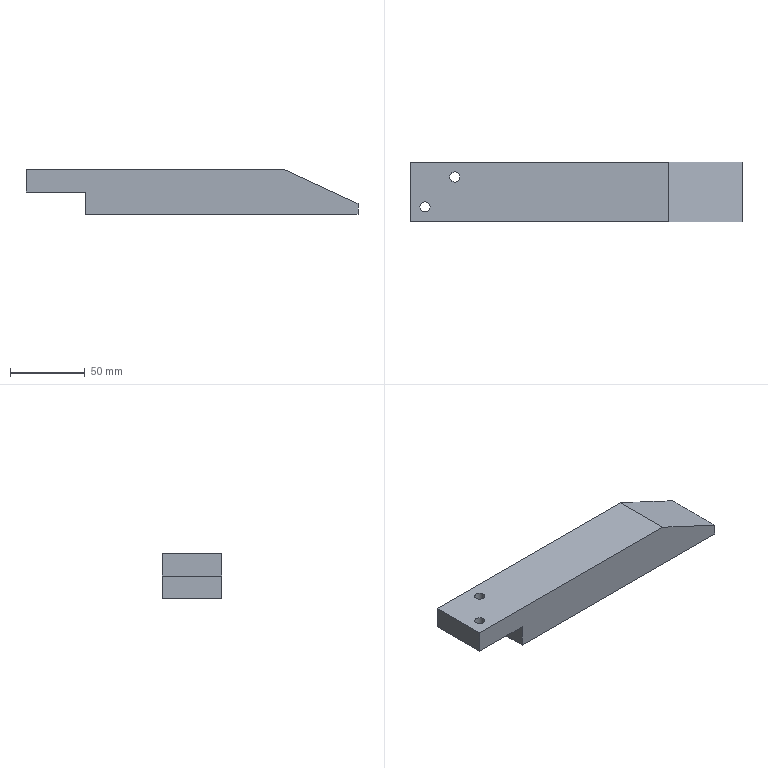Part | NX | features solid 2 | 1 solid | 11 faces | box 222 x 40 x 30 mm | volume 219063 mm3 | plane 9 | cylinder 2 | commonest cylinder face diameters 6.8 x2
STEP:
#1=CARTESIAN_POINT('',(3424.4,108.,-48.5));
#2=VERTEX_POINT('',#1);
#3=CARTESIAN_POINT('',(3421.,108.,-48.5));
#4=DIRECTION('',(0.,0.,1.));
#5=DIRECTION('',(1.,0.,0.));
#6=AXIS2_PLACEMENT_3D('',#3,#4,#5);
#7=CIRCLE('',#6,3.4);
#8=EDGE_CURVE('',#2,#2,#7,.T.);
#9=ORIENTED_EDGE('',*,*,#8,.T.);
#10=EDGE_LOOP('',(#9));
#11=FACE_BOUND('',#10,.T.);
#12=CARTESIAN_POINT('',(3444.4,128.,-48.5));
#13=VERTEX_POINT('',#12);
#14=CARTESIAN_POINT('',(3441.,128.,-48.5));
#15=DIRECTION('',(0.,0.,1.));
#16=DIRECTION('',(1.,0.,0.));
#17=AXIS2_PLACEMENT_3D('',#14,#15,#16);
#18=CIRCLE('',#17,3.4);
#19=EDGE_CURVE('',#13,#13,#18,.T.);
#20=ORIENTED_EDGE('',*,*,#19,.T.);
#21=EDGE_LOOP('',(#20));
#22=FACE_BOUND('',#21,.T.);
#23=CARTESIAN_POINT('',(3451.,138.,-48.5));
#24=VERTEX_POINT('',#23);
#25=CARTESIAN_POINT('',(3451.,98.,-48.5));
#26=VERTEX_POINT('',#25);
#27=CARTESIAN_POINT('',(3451.,0.,-48.5));
#28=DIRECTION('',(0.,-1.,0.));
#29=VECTOR('',#28,1000.);
#30=LINE('',#27,#29);
#31=EDGE_CURVE('',#24,#26,#30,.T.);
#32=ORIENTED_EDGE('',*,*,#31,.T.);
#33=CARTESIAN_POINT('',(3411.,98.,-48.5));
#34=VERTEX_POINT('',#33);
#35=CARTESIAN_POINT('',(3699.,98.,-48.5));
#36=DIRECTION('',(1.,0.,0.));
#37=VECTOR('',#36,1000.);
#38=LINE('',#35,#37);
#39=EDGE_CURVE('',#34,#26,#38,.T.);
#40=ORIENTED_EDGE('',*,*,#39,.F.);
#41=CARTESIAN_POINT('',(3411.,138.,-48.5));
#42=VERTEX_POINT('',#41);
#43=CARTESIAN_POINT('',(3411.,0.,-48.5));
#44=DIRECTION('',(0.,1.,0.));
#45=VECTOR('',#44,1000.);
#46=LINE('',#43,#45);
#47=EDGE_CURVE('',#34,#42,#46,.T.);
#48=ORIENTED_EDGE('',*,*,#47,.T.);
#49=CARTESIAN_POINT('',(3699.,138.,-48.5));
#50=DIRECTION('',(1.,0.,0.));
#51=VECTOR('',#50,1000.);
#52=LINE('',#49,#51);
#53=EDGE_CURVE('',#42,#24,#52,.T.);
#54=ORIENTED_EDGE('',*,*,#53,.T.);
#55=EDGE_LOOP('',(#32,#40,#48,#54));
#56=FACE_BOUND('',#55,.T.);
#57=CARTESIAN_POINT('',(3411.,138.,-48.5));
#58=DIRECTION('',(0.,0.,1.));
#59=DIRECTION('',(-1.,0.,0.));
#60=AXIS2_PLACEMENT_3D('',#57,#58,#59);
#61=PLANE('',#60);
#62=ADVANCED_FACE('',(#11,#22,#56),#61,.F.);
#63=CARTESIAN_POINT('',(3424.4,108.,-33.5));
#64=VERTEX_POINT('',#63);
#65=CARTESIAN_POINT('',(3421.,108.,-33.5));
#66=DIRECTION('',(0.,0.,1.));
#67=DIRECTION('',(1.,0.,0.));
#68=AXIS2_PLACEMENT_3D('',#65,#66,#67);
#69=CIRCLE('',#68,3.4);
#70=EDGE_CURVE('',#64,#64,#69,.T.);
#71=ORIENTED_EDGE('',*,*,#70,.F.);
#72=EDGE_LOOP('',(#71));
#73=FACE_BOUND('',#72,.T.);
#74=CARTESIAN_POINT('',(3444.4,128.,-33.5));
#75=VERTEX_POINT('',#74);
#76=CARTESIAN_POINT('',(3441.,128.,-33.5));
#77=DIRECTION('',(0.,0.,1.));
#78=DIRECTION('',(1.,0.,0.));
#79=AXIS2_PLACEMENT_3D('',#76,#77,#78);
#80=CIRCLE('',#79,3.4);
#81=EDGE_CURVE('',#75,#75,#80,.T.);
#82=ORIENTED_EDGE('',*,*,#81,.F.);
#83=EDGE_LOOP('',(#82));
#84=FACE_BOUND('',#83,.T.);
#85=CARTESIAN_POINT('',(3584.159,138.,-33.5));
#86=VERTEX_POINT('',#85);
#87=CARTESIAN_POINT('',(3411.,138.,-33.5));
#88=VERTEX_POINT('',#87);
#89=CARTESIAN_POINT('',(3699.,138.,-33.5));
#90=DIRECTION('',(-1.,0.,0.));
#91=VECTOR('',#90,1000.);
#92=LINE('',#89,#91);
#93=EDGE_CURVE('',#86,#88,#92,.T.);
#94=ORIENTED_EDGE('',*,*,#93,.T.);
#95=CARTESIAN_POINT('',(3411.,98.,-33.5));
#96=VERTEX_POINT('',#95);
#97=CARTESIAN_POINT('',(3411.,0.,-33.5));
#98=DIRECTION('',(0.,-1.,0.));
#99=VECTOR('',#98,1000.);
#100=LINE('',#97,#99);
#101=EDGE_CURVE('',#88,#96,#100,.T.);
#102=ORIENTED_EDGE('',*,*,#101,.T.);
#103=CARTESIAN_POINT('',(3584.159,98.,-33.5));
#104=VERTEX_POINT('',#103);
#105=CARTESIAN_POINT('',(3699.,98.,-33.5));
#106=DIRECTION('',(1.,0.,0.));
#107=VECTOR('',#106,1000.);
#108=LINE('',#105,#107);
#109=EDGE_CURVE('',#96,#104,#108,.T.);
#110=ORIENTED_EDGE('',*,*,#109,.T.);
#111=CARTESIAN_POINT('',(3584.159,118.,-33.5));
#112=DIRECTION('',(0.,-1.,0.));
#113=VECTOR('',#112,1000.);
#114=LINE('',#111,#113);
#115=EDGE_CURVE('',#86,#104,#114,.T.);
#116=ORIENTED_EDGE('',*,*,#115,.F.);
#117=EDGE_LOOP('',(#94,#102,#110,#116));
#118=FACE_BOUND('',#117,.T.);
#119=CARTESIAN_POINT('',(3699.,118.,-33.5));
#120=DIRECTION('',(0.,0.,1.));
#121=DIRECTION('',(-1.,0.,0.));
#122=AXIS2_PLACEMENT_3D('',#119,#120,#121);
#123=PLANE('',#122);
#124=ADVANCED_FACE('',(#73,#84,#118),#123,.T.);
#125=CARTESIAN_POINT('',(3633.,138.,-56.275));
#126=VERTEX_POINT('',#125);
#127=CARTESIAN_POINT('',(3642.615,138.,-60.759));
#128=DIRECTION('',(-0.9063,0.,0.4226));
#129=VECTOR('',#128,1000.);
#130=LINE('',#127,#129);
#131=EDGE_CURVE('',#126,#86,#130,.T.);
#132=ORIENTED_EDGE('',*,*,#131,.T.);
#133=ORIENTED_EDGE('',*,*,#115,.T.);
#134=CARTESIAN_POINT('',(3633.,98.,-56.275));
#135=VERTEX_POINT('',#134);
#136=CARTESIAN_POINT('',(3642.615,98.,-60.759));
#137=DIRECTION('',(0.9063,0.,-0.4226));
#138=VECTOR('',#137,1000.);
#139=LINE('',#136,#138);
#140=EDGE_CURVE('',#104,#135,#139,.T.);
#141=ORIENTED_EDGE('',*,*,#140,.T.);
#142=CARTESIAN_POINT('',(3633.,-27.,-56.275));
#143=DIRECTION('',(0.,1.,0.));
#144=VECTOR('',#143,1000.);
#145=LINE('',#142,#144);
#146=EDGE_CURVE('',#135,#126,#145,.T.);
#147=ORIENTED_EDGE('',*,*,#146,.T.);
#148=EDGE_LOOP('',(#132,#133,#141,#147));
#149=FACE_BOUND('',#148,.T.);
#150=CARTESIAN_POINT('',(3868.932,193.251,-166.292));
#151=DIRECTION('',(0.4226,0.,0.9063));
#152=DIRECTION('',(-0.9063,0.,0.4226));
#153=AXIS2_PLACEMENT_3D('',#150,#151,#152);
#154=PLANE('',#153);
#155=ADVANCED_FACE('',(#149),#154,.T.);
#156=ORIENTED_EDGE('',*,*,#47,.F.);
#157=CARTESIAN_POINT('',(3411.,98.,-53.5));
#158=DIRECTION('',(0.,0.,1.));
#159=VECTOR('',#158,1000.);
#160=LINE('',#157,#159);
#161=EDGE_CURVE('',#34,#96,#160,.T.);
#162=ORIENTED_EDGE('',*,*,#161,.T.);
#163=ORIENTED_EDGE('',*,*,#101,.F.);
#164=CARTESIAN_POINT('',(3411.,138.,-63.5));
#165=DIRECTION('',(0.,0.,1.));
#166=VECTOR('',#165,1000.);
#167=LINE('',#164,#166);
#168=EDGE_CURVE('',#42,#88,#167,.T.);
#169=ORIENTED_EDGE('',*,*,#168,.F.);
#170=EDGE_LOOP('',(#156,#162,#163,#169));
#171=FACE_BOUND('',#170,.T.);
#172=CARTESIAN_POINT('',(3411.,0.,-63.5));
#173=DIRECTION('',(-1.,0.,0.));
#174=DIRECTION('',(0.,0.,-1.));
#175=AXIS2_PLACEMENT_3D('',#172,#173,#174);
#176=PLANE('',#175);
#177=ADVANCED_FACE('',(#171),#176,.T.);
#178=ORIENTED_EDGE('',*,*,#39,.T.);
#179=CARTESIAN_POINT('',(3451.,98.,-63.5));
#180=VERTEX_POINT('',#179);
#181=CARTESIAN_POINT('',(3451.,98.,-53.5));
#182=DIRECTION('',(0.,0.,1.));
#183=VECTOR('',#182,1000.);
#184=LINE('',#181,#183);
#185=EDGE_CURVE('',#180,#26,#184,.T.);
#186=ORIENTED_EDGE('',*,*,#185,.F.);
#187=CARTESIAN_POINT('',(3633.,98.,-63.5));
#188=VERTEX_POINT('',#187);
#189=CARTESIAN_POINT('',(3699.,98.,-63.5));
#190=DIRECTION('',(-1.,0.,0.));
#191=VECTOR('',#190,1000.);
#192=LINE('',#189,#191);
#193=EDGE_CURVE('',#188,#180,#192,.T.);
#194=ORIENTED_EDGE('',*,*,#193,.F.);
#195=CARTESIAN_POINT('',(3633.,98.,-53.5));
#196=DIRECTION('',(0.,0.,-1.));
#197=VECTOR('',#196,1000.);
#198=LINE('',#195,#197);
#199=EDGE_CURVE('',#135,#188,#198,.T.);
#200=ORIENTED_EDGE('',*,*,#199,.F.);
#201=ORIENTED_EDGE('',*,*,#140,.F.);
#202=ORIENTED_EDGE('',*,*,#109,.F.);
#203=ORIENTED_EDGE('',*,*,#161,.F.);
#204=EDGE_LOOP('',(#178,#186,#194,#200,#201,#202,#203));
#205=FACE_BOUND('',#204,.T.);
#206=CARTESIAN_POINT('',(3699.,98.,-53.5));
#207=DIRECTION('',(0.,-1.,0.));
#208=DIRECTION('',(0.,0.,-1.));
#209=AXIS2_PLACEMENT_3D('',#206,#207,#208);
#210=PLANE('',#209);
#211=ADVANCED_FACE('',(#205),#210,.T.);
#212=ORIENTED_EDGE('',*,*,#53,.F.);
#213=ORIENTED_EDGE('',*,*,#168,.T.);
#214=ORIENTED_EDGE('',*,*,#93,.F.);
#215=ORIENTED_EDGE('',*,*,#131,.F.);
#216=CARTESIAN_POINT('',(3633.,138.,-63.5));
#217=VERTEX_POINT('',#216);
#218=CARTESIAN_POINT('',(3633.,138.,-53.5));
#219=DIRECTION('',(0.,0.,1.));
#220=VECTOR('',#219,1000.);
#221=LINE('',#218,#220);
#222=EDGE_CURVE('',#217,#126,#221,.T.);
#223=ORIENTED_EDGE('',*,*,#222,.F.);
#224=CARTESIAN_POINT('',(3451.,138.,-63.5));
#225=VERTEX_POINT('',#224);
#226=CARTESIAN_POINT('',(3699.,138.,-63.5));
#227=DIRECTION('',(1.,0.,0.));
#228=VECTOR('',#227,1000.);
#229=LINE('',#226,#228);
#230=EDGE_CURVE('',#225,#217,#229,.T.);
#231=ORIENTED_EDGE('',*,*,#230,.F.);
#232=CARTESIAN_POINT('',(3451.,138.,-63.5));
#233=DIRECTION('',(0.,0.,1.));
#234=VECTOR('',#233,1000.);
#235=LINE('',#232,#234);
#236=EDGE_CURVE('',#225,#24,#235,.T.);
#237=ORIENTED_EDGE('',*,*,#236,.T.);
#238=EDGE_LOOP('',(#212,#213,#214,#215,#223,#231,#237));
#239=FACE_BOUND('',#238,.T.);
#240=CARTESIAN_POINT('',(3699.,138.,-53.5));
#241=DIRECTION('',(0.,1.,0.));
#242=DIRECTION('',(0.,0.,1.));
#243=AXIS2_PLACEMENT_3D('',#240,#241,#242);
#244=PLANE('',#243);
#245=ADVANCED_FACE('',(#239),#244,.T.);
#246=ORIENTED_EDGE('',*,*,#236,.F.);
#247=CARTESIAN_POINT('',(3451.,0.,-63.5));
#248=DIRECTION('',(0.,1.,0.));
#249=VECTOR('',#248,1000.);
#250=LINE('',#247,#249);
#251=EDGE_CURVE('',#180,#225,#250,.T.);
#252=ORIENTED_EDGE('',*,*,#251,.F.);
#253=ORIENTED_EDGE('',*,*,#185,.T.);
#254=ORIENTED_EDGE('',*,*,#31,.F.);
#255=EDGE_LOOP('',(#246,#252,#253,#254));
#256=FACE_BOUND('',#255,.T.);
#257=CARTESIAN_POINT('',(3451.,0.,-63.5));
#258=DIRECTION('',(1.,0.,0.));
#259=DIRECTION('',(0.,0.,1.));
#260=AXIS2_PLACEMENT_3D('',#257,#258,#259);
#261=PLANE('',#260);
#262=ADVANCED_FACE('',(#256),#261,.F.);
#263=ORIENTED_EDGE('',*,*,#199,.T.);
#264=CARTESIAN_POINT('',(3633.,0.,-63.5));
#265=DIRECTION('',(0.,1.,0.));
#266=VECTOR('',#265,1000.);
#267=LINE('',#264,#266);
#268=EDGE_CURVE('',#188,#217,#267,.T.);
#269=ORIENTED_EDGE('',*,*,#268,.T.);
#270=ORIENTED_EDGE('',*,*,#222,.T.);
#271=ORIENTED_EDGE('',*,*,#146,.F.);
#272=EDGE_LOOP('',(#263,#269,#270,#271));
#273=FACE_BOUND('',#272,.T.);
#274=CARTESIAN_POINT('',(3633.,-27.,0.));
#275=DIRECTION('',(1.,0.,0.));
#276=DIRECTION('',(0.,0.,1.));
#277=AXIS2_PLACEMENT_3D('',#274,#275,#276);
#278=PLANE('',#277);
#279=ADVANCED_FACE('',(#273),#278,.T.);
#280=ORIENTED_EDGE('',*,*,#193,.T.);
#281=ORIENTED_EDGE('',*,*,#251,.T.);
#282=ORIENTED_EDGE('',*,*,#230,.T.);
#283=ORIENTED_EDGE('',*,*,#268,.F.);
#284=EDGE_LOOP('',(#280,#281,#282,#283));
#285=FACE_BOUND('',#284,.T.);
#286=CARTESIAN_POINT('',(3421.,0.,-63.5));
#287=DIRECTION('',(0.,0.,-1.));
#288=DIRECTION('',(1.,0.,0.));
#289=AXIS2_PLACEMENT_3D('',#286,#287,#288);
#290=PLANE('',#289);
#291=ADVANCED_FACE('',(#285),#290,.T.);
#292=ORIENTED_EDGE('',*,*,#81,.T.);
#293=EDGE_LOOP('',(#292));
#294=FACE_BOUND('',#293,.T.);
#295=ORIENTED_EDGE('',*,*,#19,.F.);
#296=EDGE_LOOP('',(#295));
#297=FACE_BOUND('',#296,.T.);
#298=CARTESIAN_POINT('',(3441.,128.,-48.5));
#299=DIRECTION('',(0.,0.,1.));
#300=DIRECTION('',(-1.,0.,0.));
#301=AXIS2_PLACEMENT_3D('',#298,#299,#300);
#302=CYLINDRICAL_SURFACE('',#301,3.4);
#303=ADVANCED_FACE('',(#294,#297),#302,.F.);
#304=ORIENTED_EDGE('',*,*,#70,.T.);
#305=EDGE_LOOP('',(#304));
#306=FACE_BOUND('',#305,.T.);
#307=ORIENTED_EDGE('',*,*,#8,.F.);
#308=EDGE_LOOP('',(#307));
#309=FACE_BOUND('',#308,.T.);
#310=CARTESIAN_POINT('',(3421.,108.,-48.5));
#311=DIRECTION('',(0.,0.,1.));
#312=DIRECTION('',(-1.,0.,0.));
#313=AXIS2_PLACEMENT_3D('',#310,#311,#312);
#314=CYLINDRICAL_SURFACE('',#313,3.4);
#315=ADVANCED_FACE('',(#306,#309),#314,.F.);
#316=CLOSED_SHELL('',(#62,#124,#155,#177,#211,#245,#262,#279,#291,#303,#315));
#317=MANIFOLD_SOLID_BREP('',#316);
#318=(LENGTH_UNIT()NAMED_UNIT(*)SI_UNIT(.MILLI.,.METRE.));
#319=UNCERTAINTY_MEASURE_WITH_UNIT(LENGTH_MEASURE(0.00001),#318,'','');
#320=(NAMED_UNIT(*)PLANE_ANGLE_UNIT()SI_UNIT($,.RADIAN.));
#321=(NAMED_UNIT(*)SI_UNIT($,.STERADIAN.)SOLID_ANGLE_UNIT());
#322=(GEOMETRIC_REPRESENTATION_CONTEXT(3)GLOBAL_UNCERTAINTY_ASSIGNED_CONTEXT((#319))GLOBAL_UNIT_ASSIGNED_CONTEXT((#318,#320,#321))REPRESENTATION_CONTEXT('',''));
#323=ADVANCED_BREP_SHAPE_REPRESENTATION('',(#317),#322);